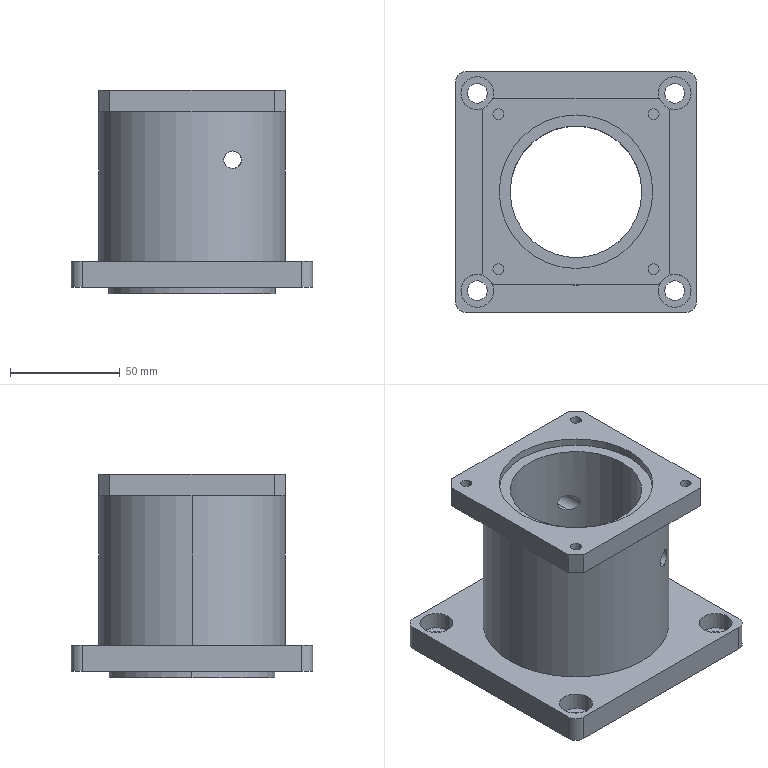Part | NX | features BREP 1 | 1 solid | 65 faces | box 110 x 110 x 93 mm | volume 340709 mm3 | cylinder 40 | plane 25 | commonest cylinder face diameters 5 x8 9 x8 15 x8 8 x4 10 x4 60 x2